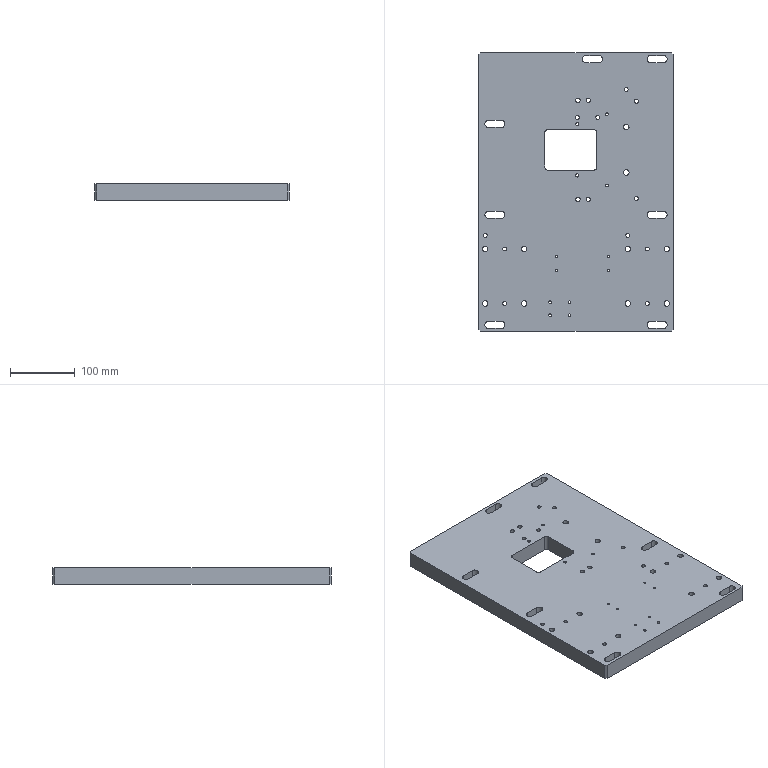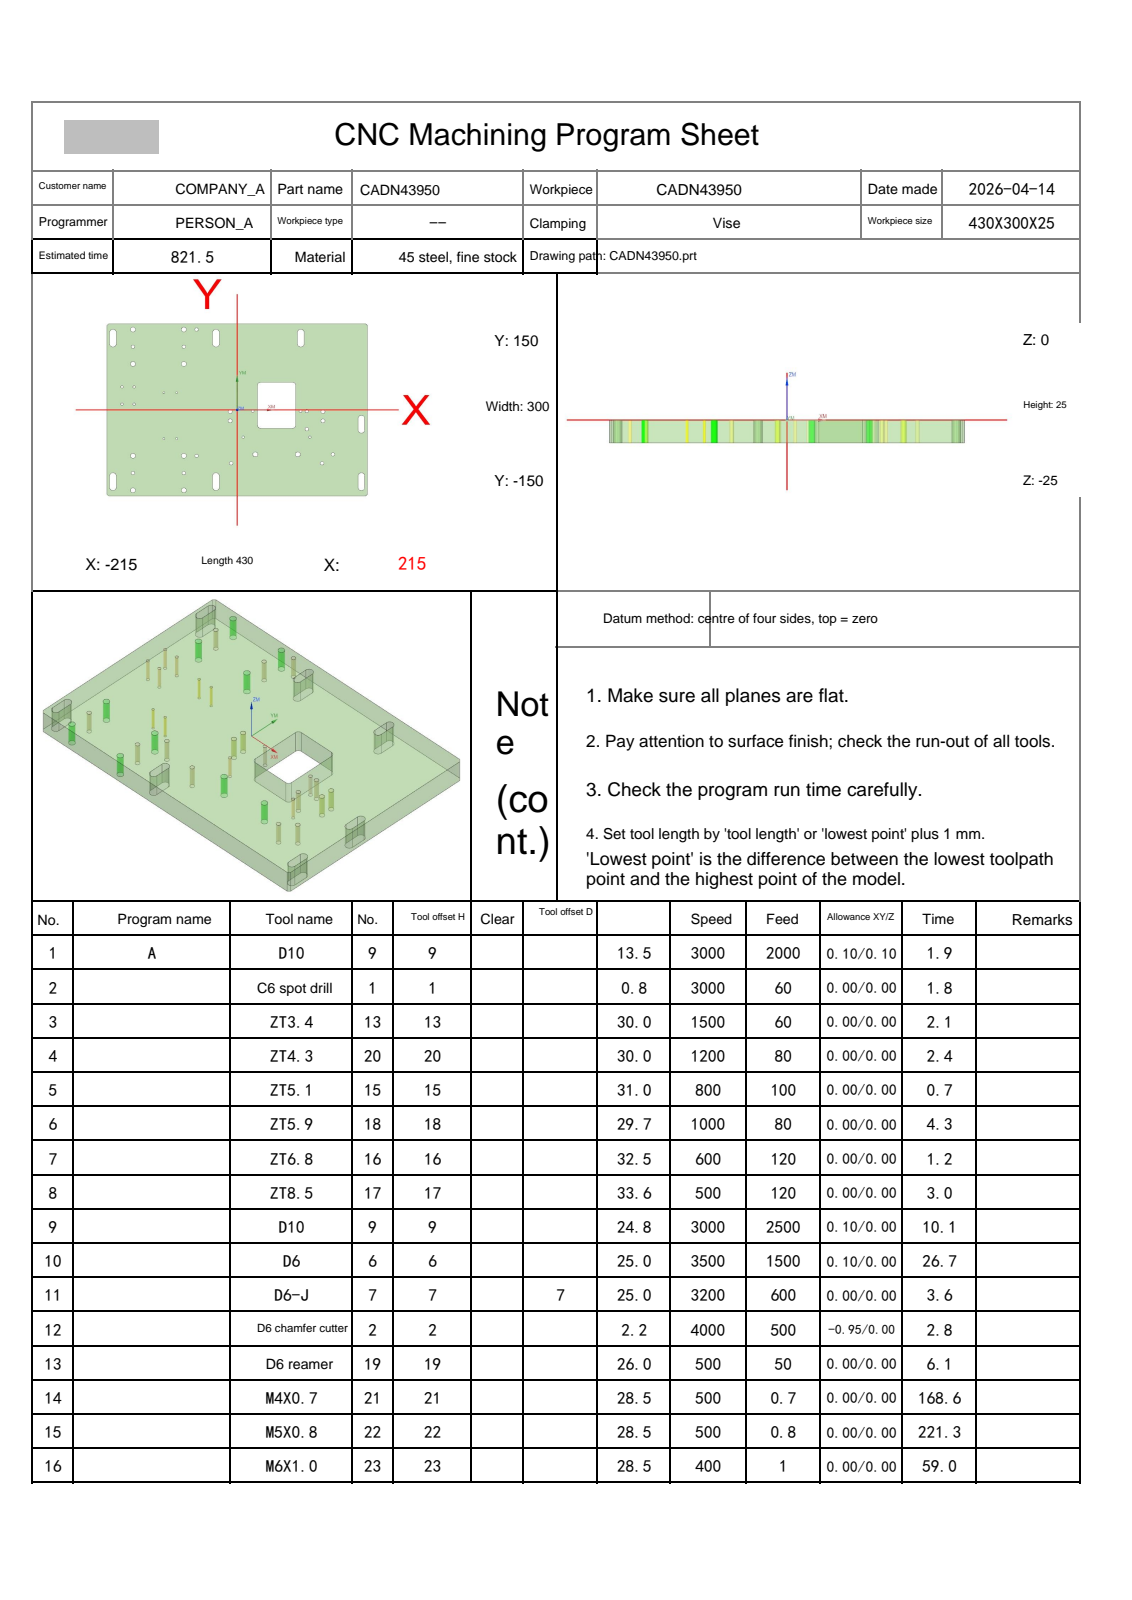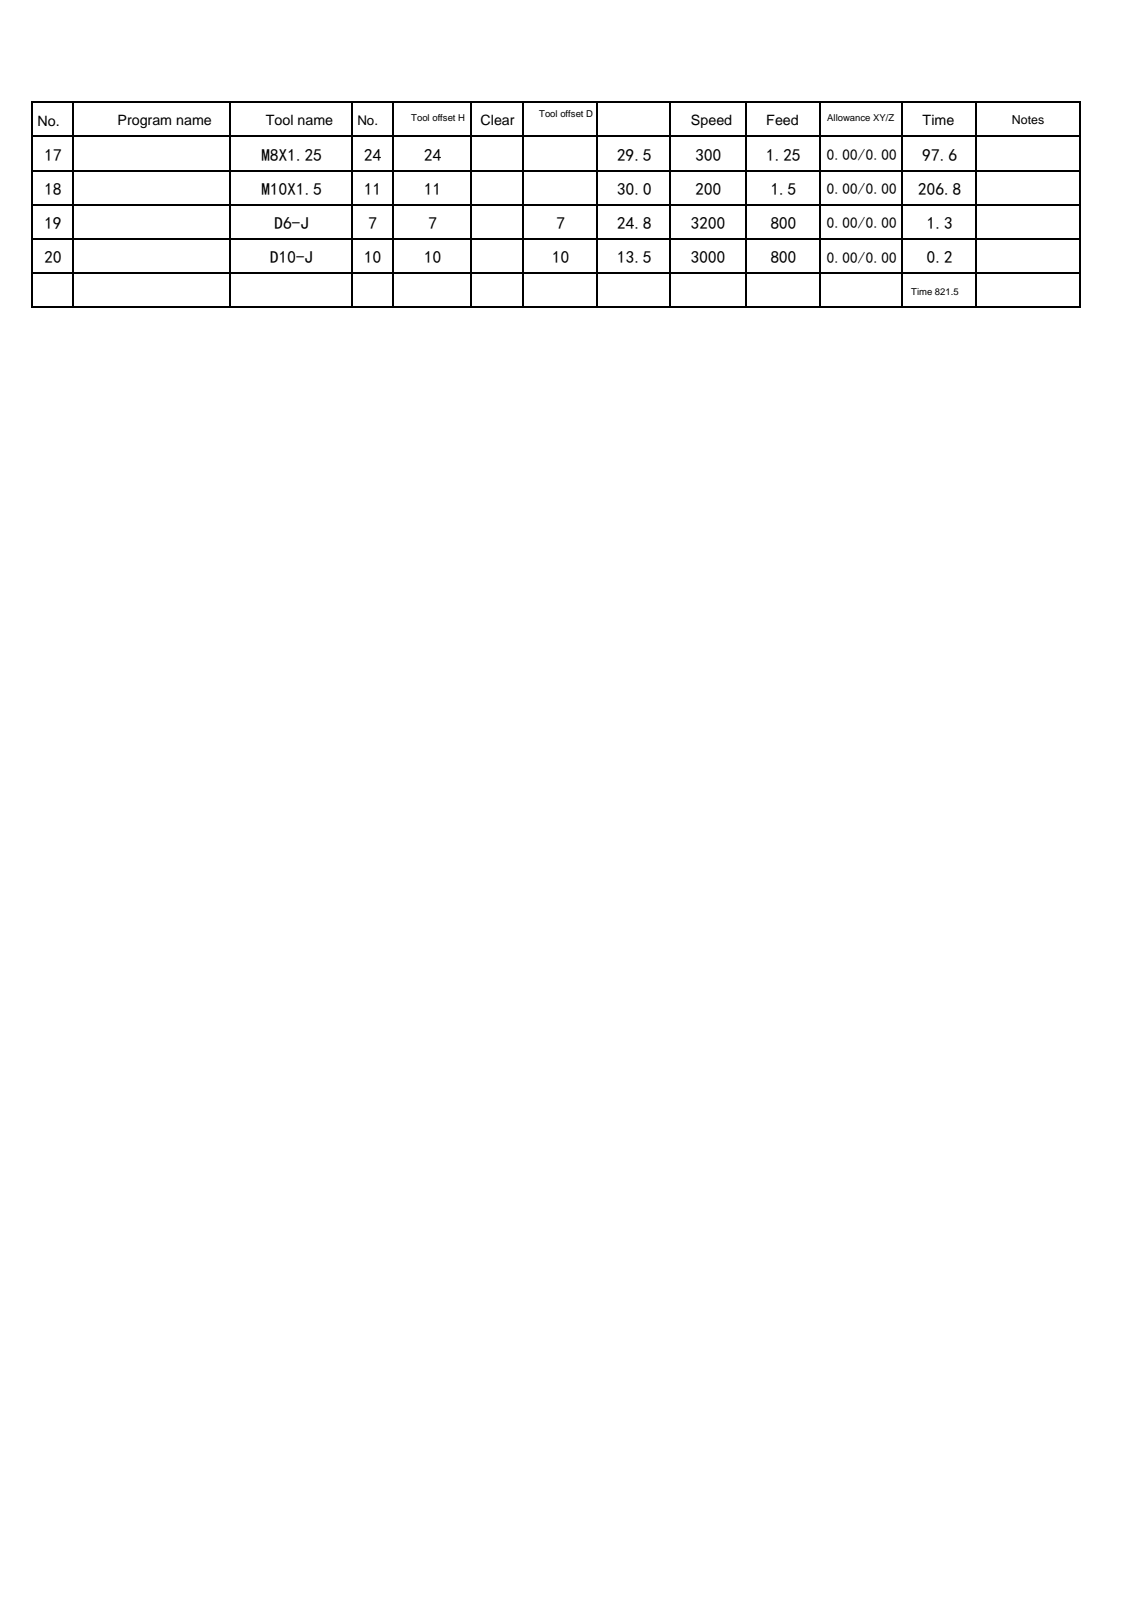NC program | NX | posted by the shop | part box 300 x 430 x 25 mm
Lines 1269 to 2074 of 7024:
N10 T06 M06
(D6  D=6. R=0. H=06 ce=0.10 di=0.00)
G00 G90 G54 X-207.4 Y-125. M03 S3500
G43 H06 Z20.
M08
Z.5
G01 Y-135. Z.455 F1500.
G03 X-205. Y-137.4 Z.438 I2.4 J0.0
X-202.6 Y-135. Z.421 I0.0 J2.4
G01 Y-115. Z.331
G03 X-205. Y-112.6 Z.314 I-2.4 J0.0
X-207.4 Y-115. Z.297 I0.0 J-2.4
G01 Y-135. Z.207
G03 X-205. Y-137.4 Z.191 I2.4 J0.0
X-202.6 Y-135. Z.174 I0.0 J2.4
G01 Y-115. Z.084
G03 X-205. Y-112.6 Z.067 I-2.4 J0.0
X-207.4 Y-115. Z.05 I0.0 J-2.4
G01 Y-135. Z-.04
G03 X-205. Y-137.4 Z-.057 I2.4 J0.0
X-202.6 Y-135. Z-.074 I0.0 J2.4
G01 Y-115. Z-.164
G03 X-205. Y-112.6 Z-.181 I-2.4 J0.0
X-207.4 Y-115. Z-.198 I0.0 J-2.4
G01 Y-135. Z-.288
G03 X-205. Y-137.4 Z-.305 I2.4 J0.0
X-202.6 Y-135. Z-.322 I0.0 J2.4
G01 Y-115. Z-.411
G03 X-205. Y-112.6 Z-.428 I-2.4 J0.0
X-207.4 Y-115. Z-.445 I0.0 J-2.4
G01 Y-135. Z-.535
G03 X-205. Y-137.4 Z-.552 I2.4 J0.0
X-202.6 Y-135. Z-.569 I0.0 J2.4
G01 Y-115. Z-.659
G03 X-205. Y-112.6 Z-.676 I-2.4 J0.0
X-207.4 Y-115. Z-.693 I0.0 J-2.4
G01 Y-135. Z-.783
G03 X-205. Y-137.4 Z-.8 I2.4 J0.0
X-202.6 Y-135. Z-.817 I0.0 J2.4
G01 Y-115. Z-.907
G03 X-205. Y-112.6 Z-.924 I-2.4 J0.0
X-207.4 Y-115. Z-.94 I0.0 J-2.4
G01 Y-135. Z-1.03
G03 X-205. Y-137.4 Z-1.047 I2.4 J0.0
X-202.6 Y-135. Z-1.064 I0.0 J2.4
G01 Y-115. Z-1.154
G03 X-205. Y-112.6 Z-1.171 I-2.4 J0.0
X-207.4 Y-115. Z-1.188 I0.0 J-2.4
G01 Y-135. Z-1.278
G03 X-205. Y-137.4 Z-1.295 I2.4 J0.0
X-202.6 Y-135. Z-1.312 I0.0 J2.4
G01 Y-115. Z-1.402
G03 X-205. Y-112.6 Z-1.419 I-2.4 J0.0
X-207.4 Y-115. Z-1.436 I0.0 J-2.4
G01 Y-135. Z-1.526
G03 X-205. Y-137.4 Z-1.542 I2.4 J0.0
X-202.6 Y-135. Z-1.559 I0.0 J2.4
G01 Y-115. Z-1.649
G03 X-205. Y-112.6 Z-1.666 I-2.4 J0.0
X-207.4 Y-115. Z-1.683 I0.0 J-2.4
G01 Y-135. Z-1.773
G03 X-205. Y-137.4 Z-1.79 I2.4 J0.0
X-202.6 Y-135. Z-1.807 I0.0 J2.4
G01 Y-115. Z-1.897
G03 X-205. Y-112.6 Z-1.914 I-2.4 J0.0
X-207.4 Y-115. Z-1.931 I0.0 J-2.4
G01 Y-135. Z-2.021
G03 X-205. Y-137.4 Z-2.038 I2.4 J0.0
X-202.6 Y-135. Z-2.055 I0.0 J2.4
G01 Y-115. Z-2.144
G03 X-205. Y-112.6 Z-2.161 I-2.4 J0.0
X-207.4 Y-115. Z-2.178 I0.0 J-2.4
G01 Y-135. Z-2.268
G03 X-205. Y-137.4 Z-2.285 I2.4 J0.0
X-202.6 Y-135. Z-2.302 I0.0 J2.4
G01 Y-115. Z-2.392
G03 X-205. Y-112.6 Z-2.409 I-2.4 J0.0
X-207.4 Y-115. Z-2.426 I0.0 J-2.4
G01 Y-135. Z-2.516
G03 X-205. Y-137.4 Z-2.533 I2.4 J0.0
X-202.6 Y-135. Z-2.55 I0.0 J2.4
G01 Y-115. Z-2.64
G03 X-205. Y-112.6 Z-2.657 I-2.4 J0.0
X-207.4 Y-115. Z-2.673 I0.0 J-2.4
G01 Y-135. Z-2.763
G03 X-205. Y-137.4 Z-2.78 I2.4 J0.0
X-202.6 Y-135. Z-2.797 I0.0 J2.4
G01 Y-115. Z-2.887
G03 X-205. Y-112.6 Z-2.904 I-2.4 J0.0
X-207.4 Y-115. Z-2.921 I0.0 J-2.4
G01 Y-135. Z-3.011
G03 X-205. Y-137.4 Z-3.028 I2.4 J0.0
X-202.6 Y-135. Z-3.045 I0.0 J2.4
G01 Y-115. Z-3.135
G03 X-205. Y-112.6 Z-3.152 I-2.4 J0.0
X-207.4 Y-115. Z-3.169 I0.0 J-2.4
G01 Y-135. Z-3.259
G03 X-205. Y-137.4 Z-3.275 I2.4 J0.0
X-202.6 Y-135. Z-3.292 I0.0 J2.4
G01 Y-115. Z-3.382
G03 X-205. Y-112.6 Z-3.399 I-2.4 J0.0
X-207.4 Y-115. Z-3.416 I0.0 J-2.4
G01 Y-135. Z-3.506
G03 X-205. Y-137.4 Z-3.523 I2.4 J0.0
X-202.6 Y-135. Z-3.54 I0.0 J2.4
G01 Y-115. Z-3.63
G03 X-205. Y-112.6 Z-3.647 I-2.4 J0.0
X-207.4 Y-115. Z-3.664 I0.0 J-2.4
G01 Y-135. Z-3.754
G03 X-205. Y-137.4 Z-3.771 I2.4 J0.0
X-202.6 Y-135. Z-3.788 I0.0 J2.4
G01 Y-115. Z-3.877
G03 X-205. Y-112.6 Z-3.894 I-2.4 J0.0
X-207.4 Y-115. Z-3.911 I0.0 J-2.4
G01 Y-135. Z-4.001
G03 X-205. Y-137.4 Z-4.018 I2.4 J0.0
X-202.6 Y-135. Z-4.035 I0.0 J2.4
G01 Y-115. Z-4.125
G03 X-205. Y-112.6 Z-4.142 I-2.4 J0.0
X-207.4 Y-115. Z-4.159 I0.0 J-2.4
G01 Y-135. Z-4.249
G03 X-205. Y-137.4 Z-4.266 I2.4 J0.0
X-202.6 Y-135. Z-4.283 I0.0 J2.4
G01 Y-115. Z-4.373
G03 X-205. Y-112.6 Z-4.39 I-2.4 J0.0
X-207.4 Y-115. Z-4.407 I0.0 J-2.4
G01 Y-135. Z-4.496
G03 X-205. Y-137.4 Z-4.513 I2.4 J0.0
X-202.6 Y-135. Z-4.53 I0.0 J2.4
G01 Y-115. Z-4.62
G03 X-205. Y-112.6 Z-4.637 I-2.4 J0.0
X-207.4 Y-115. Z-4.654 I0.0 J-2.4
G01 Y-135. Z-4.744
G03 X-205. Y-137.4 Z-4.761 I2.4 J0.0
X-202.6 Y-135. Z-4.778 I0.0 J2.4
G01 Y-115. Z-4.868
G03 X-205. Y-112.6 Z-4.885 I-2.4 J0.0
X-207.4 Y-115. Z-4.902 I0.0 J-2.4
G01 Y-135. Z-4.992
G03 X-205. Y-137.4 Z-5.008 I2.4 J0.0
X-202.6 Y-135. Z-5.025 I0.0 J2.4
G01 Y-115. Z-5.115
G03 X-205. Y-112.6 Z-5.132 I-2.4 J0.0
X-207.4 Y-115. Z-5.149 I0.0 J-2.4
G01 Y-135. Z-5.239
G03 X-205. Y-137.4 Z-5.256 I2.4 J0.0
X-202.6 Y-135. Z-5.273 I0.0 J2.4
G01 Y-115. Z-5.363
G03 X-205. Y-112.6 Z-5.38 I-2.4 J0.0
X-207.4 Y-115. Z-5.397 I0.0 J-2.4
G01 Y-135. Z-5.487
G03 X-205. Y-137.4 Z-5.504 I2.4 J0.0
X-202.6 Y-135. Z-5.521 I0.0 J2.4
G01 Y-115. Z-5.61
G03 X-205. Y-112.6 Z-5.627 I-2.4 J0.0
X-207.4 Y-115. Z-5.644 I0.0 J-2.4
G01 Y-135. Z-5.734
G03 X-205. Y-137.4 Z-5.751 I2.4 J0.0
X-202.6 Y-135. Z-5.768 I0.0 J2.4
G01 Y-115. Z-5.858
G03 X-205. Y-112.6 Z-5.875 I-2.4 J0.0
X-207.4 Y-115. Z-5.892 I0.0 J-2.4
G01 Y-135. Z-5.982
G03 X-205. Y-137.4 Z-5.999 I2.4 J0.0
X-202.6 Y-135. Z-6.016 I0.0 J2.4
G01 Y-115. Z-6.106
G03 X-205. Y-112.6 Z-6.123 I-2.4 J0.0
X-207.4 Y-115. Z-6.14 I0.0 J-2.4
G01 Y-135. Z-6.229
G03 X-205. Y-137.4 Z-6.246 I2.4 J0.0
X-202.6 Y-135. Z-6.263 I0.0 J2.4
G01 Y-115. Z-6.353
G03 X-205. Y-112.6 Z-6.37 I-2.4 J0.0
X-207.4 Y-115. Z-6.387 I0.0 J-2.4
G01 Y-135. Z-6.477
G03 X-205. Y-137.4 Z-6.494 I2.4 J0.0
X-202.6 Y-135. Z-6.511 I0.0 J2.4
G01 Y-115. Z-6.601
G03 X-205. Y-112.6 Z-6.618 I-2.4 J0.0
X-207.4 Y-115. Z-6.635 I0.0 J-2.4
G01 Y-135. Z-6.725
G03 X-205. Y-137.4 Z-6.742 I2.4 J0.0
X-202.6 Y-135. Z-6.758 I0.0 J2.4
G01 Y-115. Z-6.848
G03 X-205. Y-112.6 Z-6.865 I-2.4 J0.0
X-207.4 Y-115. Z-6.882 I0.0 J-2.4
G01 Y-135. Z-6.972
G03 X-205. Y-137.4 Z-6.989 I2.4 J0.0
X-202.6 Y-135. Z-7.006 I0.0 J2.4
G01 Y-115. Z-7.096
G03 X-205. Y-112.6 Z-7.113 I-2.4 J0.0
X-207.4 Y-115. Z-7.13 I0.0 J-2.4
G01 Y-135. Z-7.22
G03 X-205. Y-137.4 Z-7.237 I2.4 J0.0
X-202.6 Y-135. Z-7.254 I0.0 J2.4
G01 Y-115. Z-7.343
G03 X-205. Y-112.6 Z-7.36 I-2.4 J0.0
X-207.4 Y-115. Z-7.377 I0.0 J-2.4
G01 Y-135. Z-7.467
G03 X-205. Y-137.4 Z-7.484 I2.4 J0.0
X-202.6 Y-135. Z-7.501 I0.0 J2.4
G01 Y-115. Z-7.591
G03 X-205. Y-112.6 Z-7.608 I-2.4 J0.0
X-207.4 Y-115. Z-7.625 I0.0 J-2.4
G01 Y-135. Z-7.715
G03 X-205. Y-137.4 Z-7.732 I2.4 J0.0
X-202.6 Y-135. Z-7.749 I0.0 J2.4
G01 Y-115. Z-7.839
G03 X-205. Y-112.6 Z-7.856 I-2.4 J0.0
X-207.4 Y-115. Z-7.873 I0.0 J-2.4
G01 Y-135. Z-7.962
G03 X-205. Y-137.4 Z-7.979 I2.4 J0.0
X-202.6 Y-135. Z-7.996 I0.0 J2.4
G01 Y-115. Z-8.086
G03 X-205. Y-112.6 Z-8.103 I-2.4 J0.0
X-207.4 Y-115. Z-8.12 I0.0 J-2.4
G01 Y-135. Z-8.21
G03 X-205. Y-137.4 Z-8.227 I2.4 J0.0
X-202.6 Y-135. Z-8.244 I0.0 J2.4
G01 Y-115. Z-8.334
G03 X-205. Y-112.6 Z-8.351 I-2.4 J0.0
X-207.4 Y-115. Z-8.368 I0.0 J-2.4
G01 Y-135. Z-8.458
G03 X-205. Y-137.4 Z-8.475 I2.4 J0.0
X-202.6 Y-135. Z-8.491 I0.0 J2.4
G01 Y-115. Z-8.581
G03 X-205. Y-112.6 Z-8.598 I-2.4 J0.0
X-207.4 Y-115. Z-8.615 I0.0 J-2.4
G01 Y-135. Z-8.705
G03 X-205. Y-137.4 Z-8.722 I2.4 J0.0
X-202.6 Y-135. Z-8.739 I0.0 J2.4
G01 Y-115. Z-8.829
G03 X-205. Y-112.6 Z-8.846 I-2.4 J0.0
X-207.4 Y-115. Z-8.863 I0.0 J-2.4
G01 Y-135. Z-8.953
G03 X-205. Y-137.4 Z-8.97 I2.4 J0.0
X-202.6 Y-135. Z-8.987 I0.0 J2.4
G01 Y-115. Z-9.077
G03 X-205. Y-112.6 Z-9.093 I-2.4 J0.0
X-207.4 Y-115. Z-9.11 I0.0 J-2.4
G01 Y-135. Z-9.2
G03 X-205. Y-137.4 Z-9.217 I2.4 J0.0
X-202.6 Y-135. Z-9.234 I0.0 J2.4
G01 Y-115. Z-9.324
G03 X-205. Y-112.6 Z-9.341 I-2.4 J0.0
X-207.4 Y-115. Z-9.358 I0.0 J-2.4
G01 Y-135. Z-9.448
G03 X-205. Y-137.4 Z-9.465 I2.4 J0.0
X-202.6 Y-135. Z-9.482 I0.0 J2.4
G01 Y-115. Z-9.572
G03 X-205. Y-112.6 Z-9.589 I-2.4 J0.0
X-207.4 Y-115. Z-9.606 I0.0 J-2.4
G01 Y-135. Z-9.695
G03 X-205. Y-137.4 Z-9.712 I2.4 J0.0
X-202.6 Y-135. Z-9.729 I0.0 J2.4
G01 Y-115. Z-9.819
G03 X-205. Y-112.6 Z-9.836 I-2.4 J0.0
X-207.4 Y-115. Z-9.853 I0.0 J-2.4
G01 Y-135. Z-9.943
G03 X-205. Y-137.4 Z-9.96 I2.4 J0.0
X-202.6 Y-135. Z-9.977 I0.0 J2.4
G01 Y-115. Z-10.067
G03 X-205. Y-112.6 Z-10.084 I-2.4 J0.0
X-207.4 Y-115. Z-10.101 I0.0 J-2.4
G01 Y-135. Z-10.191
G03 X-205. Y-137.4 Z-10.208 I2.4 J0.0
X-202.6 Y-135. Z-10.224 I0.0 J2.4
G01 Y-115. Z-10.314
G03 X-205. Y-112.6 Z-10.331 I-2.4 J0.0
X-207.4 Y-115. Z-10.348 I0.0 J-2.4
G01 Y-135. Z-10.438
G03 X-205. Y-137.4 Z-10.455 I2.4 J0.0
X-202.6 Y-135. Z-10.472 I0.0 J2.4
G01 Y-115. Z-10.562
G03 X-205. Y-112.6 Z-10.579 I-2.4 J0.0
X-207.4 Y-115. Z-10.596 I0.0 J-2.4
G01 Y-135. Z-10.686
G03 X-205. Y-137.4 Z-10.703 I2.4 J0.0
X-202.6 Y-135. Z-10.72 I0.0 J2.4
G01 Y-115. Z-10.81
G03 X-205. Y-112.6 Z-10.826 I-2.4 J0.0
X-207.4 Y-115. Z-10.843 I0.0 J-2.4
G01 Y-135. Z-10.933
G03 X-205. Y-137.4 Z-10.95 I2.4 J0.0
X-202.6 Y-135. Z-10.967 I0.0 J2.4
G01 Y-115. Z-11.057
G03 X-205. Y-112.6 Z-11.074 I-2.4 J0.0
X-207.4 Y-115. Z-11.091 I0.0 J-2.4
G01 Y-135. Z-11.181
G03 X-205. Y-137.4 Z-11.198 I2.4 J0.0
X-202.6 Y-135. Z-11.215 I0.0 J2.4
G01 Y-115. Z-11.305
G03 X-205. Y-112.6 Z-11.322 I-2.4 J0.0
X-207.4 Y-115. Z-11.339 I0.0 J-2.4
G01 Y-135. Z-11.428
G03 X-205. Y-137.4 Z-11.445 I2.4 J0.0
X-202.6 Y-135. Z-11.462 I0.0 J2.4
G01 Y-115. Z-11.552
G03 X-205. Y-112.6 Z-11.569 I-2.4 J0.0
X-207.4 Y-115. Z-11.586 I0.0 J-2.4
G01 Y-135. Z-11.676
G03 X-205. Y-137.4 Z-11.693 I2.4 J0.0
X-202.6 Y-135. Z-11.71 I0.0 J2.4
G01 Y-115. Z-11.8
G03 X-205. Y-112.6 Z-11.817 I-2.4 J0.0
X-207.4 Y-115. Z-11.834 I0.0 J-2.4
G01 Y-135. Z-11.924
G03 X-205. Y-137.4 Z-11.941 I2.4 J0.0
X-202.6 Y-135. Z-11.957 I0.0 J2.4
G01 Y-115. Z-12.047
G03 X-205. Y-112.6 Z-12.064 I-2.4 J0.0
X-207.4 Y-115. Z-12.081 I0.0 J-2.4
G01 Y-135. Z-12.171
G03 X-205. Y-137.4 Z-12.188 I2.4 J0.0
X-202.6 Y-135. Z-12.205 I0.0 J2.4
G01 Y-115. Z-12.295
G03 X-205. Y-112.6 Z-12.312 I-2.4 J0.0
X-207.4 Y-115. Z-12.329 I0.0 J-2.4
G01 Y-135. Z-12.419
G03 X-205. Y-137.4 Z-12.436 I2.4 J0.0
X-202.6 Y-135. Z-12.453 I0.0 J2.4
G01 Y-115. Z-12.543
G03 X-205. Y-112.6 Z-12.559 I-2.4 J0.0
X-207.4 Y-115. Z-12.576 I0.0 J-2.4
G01 Y-135. Z-12.666
G03 X-205. Y-137.4 Z-12.683 I2.4 J0.0
X-202.6 Y-135. Z-12.7 I0.0 J2.4
G01 Y-115. Z-12.79
G03 X-205. Y-112.6 Z-12.807 I-2.4 J0.0
X-207.4 Y-115. Z-12.824 I0.0 J-2.4
G01 Y-135. Z-12.914
G03 X-205. Y-137.4 Z-12.931 I2.4 J0.0
X-202.6 Y-135. Z-12.948 I0.0 J2.4
G01 Y-115. Z-13.038
G03 X-205. Y-112.6 Z-13.055 I-2.4 J0.0
X-207.4 Y-115. Z-13.072 I0.0 J-2.4
G01 Y-135. Z-13.161
G03 X-205. Y-137.4 Z-13.178 I2.4 J0.0
X-202.6 Y-135. Z-13.195 I0.0 J2.4
G01 Y-115. Z-13.285
G03 X-205. Y-112.6 Z-13.302 I-2.4 J0.0
X-207.4 Y-115. Z-13.319 I0.0 J-2.4
G01 Y-135. Z-13.409
G03 X-205. Y-137.4 Z-13.426 I2.4 J0.0
X-202.6 Y-135. Z-13.443 I0.0 J2.4
G01 Y-115. Z-13.533
G03 X-205. Y-112.6 Z-13.55 I-2.4 J0.0
X-207.4 Y-115. Z-13.567 I0.0 J-2.4
G01 Y-135. Z-13.657
G03 X-205. Y-137.4 Z-13.674 I2.4 J0.0
X-202.6 Y-135. Z-13.69 I0.0 J2.4
G01 Y-115. Z-13.78
G03 X-205. Y-112.6 Z-13.797 I-2.4 J0.0
X-207.4 Y-115. Z-13.814 I0.0 J-2.4
G01 Y-135. Z-13.904
G03 X-205. Y-137.4 Z-13.921 I2.4 J0.0
X-202.6 Y-135. Z-13.938 I0.0 J2.4
G01 Y-115. Z-14.028
G03 X-205. Y-112.6 Z-14.045 I-2.4 J0.0
X-207.4 Y-115. Z-14.062 I0.0 J-2.4
G01 Y-135. Z-14.152
G03 X-205. Y-137.4 Z-14.169 I2.4 J0.0
X-202.6 Y-135. Z-14.186 I0.0 J2.4
G01 Y-115. Z-14.276
G03 X-205. Y-112.6 Z-14.292 I-2.4 J0.0
X-207.4 Y-115. Z-14.309 I0.0 J-2.4
G01 Y-135. Z-14.399
G03 X-205. Y-137.4 Z-14.416 I2.4 J0.0
X-202.6 Y-135. Z-14.433 I0.0 J2.4
G01 Y-115. Z-14.523
G03 X-205. Y-112.6 Z-14.54 I-2.4 J0.0
X-207.4 Y-115. Z-14.557 I0.0 J-2.4
G01 Y-135. Z-14.647
G03 X-205. Y-137.4 Z-14.664 I2.4 J0.0
X-202.6 Y-135. Z-14.681 I0.0 J2.4
G01 Y-115. Z-14.771
G03 X-205. Y-112.6 Z-14.788 I-2.4 J0.0
X-207.4 Y-115. Z-14.805 I0.0 J-2.4
G01 Y-135. Z-14.894
G03 X-205. Y-137.4 Z-14.911 I2.4 J0.0
X-202.6 Y-135. Z-14.928 I0.0 J2.4
G01 Y-115. Z-15.018
G03 X-205. Y-112.6 Z-15.035 I-2.4 J0.0
X-207.4 Y-115. Z-15.052 I0.0 J-2.4
G01 Y-135. Z-15.142
G03 X-205. Y-137.4 Z-15.159 I2.4 J0.0
X-202.6 Y-135. Z-15.176 I0.0 J2.4
G01 Y-115. Z-15.266
G03 X-205. Y-112.6 Z-15.283 I-2.4 J0.0
X-207.4 Y-115. Z-15.3 I0.0 J-2.4
G01 Y-135. Z-15.39
G03 X-205. Y-137.4 Z-15.407 I2.4 J0.0
X-202.6 Y-135. Z-15.423 I0.0 J2.4
G01 Y-115. Z-15.513
G03 X-205. Y-112.6 Z-15.53 I-2.4 J0.0
X-207.4 Y-115. Z-15.547 I0.0 J-2.4
G01 Y-135. Z-15.637
G03 X-205. Y-137.4 Z-15.654 I2.4 J0.0
X-202.6 Y-135. Z-15.671 I0.0 J2.4
G01 Y-115. Z-15.761
G03 X-205. Y-112.6 Z-15.778 I-2.4 J0.0
X-207.4 Y-115. Z-15.795 I0.0 J-2.4
G01 Y-135. Z-15.885
G03 X-205. Y-137.4 Z-15.902 I2.4 J0.0
X-202.6 Y-135. Z-15.919 I0.0 J2.4
G01 Y-115. Z-16.009
G03 X-205. Y-112.6 Z-16.025 I-2.4 J0.0
X-207.4 Y-115. Z-16.042 I0.0 J-2.4
G01 Y-135. Z-16.132
G03 X-205. Y-137.4 Z-16.149 I2.4 J0.0
X-202.6 Y-135. Z-16.166 I0.0 J2.4
G01 Y-115. Z-16.256
G03 X-205. Y-112.6 Z-16.273 I-2.4 J0.0
X-207.4 Y-115. Z-16.29 I0.0 J-2.4
G01 Y-135. Z-16.38
G03 X-205. Y-137.4 Z-16.397 I2.4 J0.0
X-202.6 Y-135. Z-16.414 I0.0 J2.4
G01 Y-115. Z-16.504
G03 X-205. Y-112.6 Z-16.521 I-2.4 J0.0
X-207.4 Y-115. Z-16.538 I0.0 J-2.4
G01 Y-135. Z-16.627
G03 X-205. Y-137.4 Z-16.644 I2.4 J0.0
X-202.6 Y-135. Z-16.661 I0.0 J2.4
G01 Y-115. Z-16.751
G03 X-205. Y-112.6 Z-16.768 I-2.4 J0.0
X-207.4 Y-115. Z-16.785 I0.0 J-2.4
G01 Y-135. Z-16.875
G03 X-205. Y-137.4 Z-16.892 I2.4 J0.0
X-202.6 Y-135. Z-16.909 I0.0 J2.4
G01 Y-115. Z-16.999
G03 X-205. Y-112.6 Z-17.016 I-2.4 J0.0
X-207.4 Y-115. Z-17.033 I0.0 J-2.4
G01 Y-135. Z-17.123
G03 X-205. Y-137.4 Z-17.14 I2.4 J0.0
X-202.6 Y-135. Z-17.157 I0.0 J2.4
G01 Y-115. Z-17.246
G03 X-205. Y-112.6 Z-17.263 I-2.4 J0.0
X-207.4 Y-115. Z-17.28 I0.0 J-2.4
G01 Y-135. Z-17.37
G03 X-205. Y-137.4 Z-17.387 I2.4 J0.0
X-202.6 Y-135. Z-17.404 I0.0 J2.4
G01 Y-115. Z-17.494
G03 X-205. Y-112.6 Z-17.511 I-2.4 J0.0
X-207.4 Y-115. Z-17.528 I0.0 J-2.4
G01 Y-135. Z-17.618
G03 X-205. Y-137.4 Z-17.635 I2.4 J0.0
X-202.6 Y-135. Z-17.652 I0.0 J2.4
G01 Y-115. Z-17.742
G03 X-205. Y-112.6 Z-17.758 I-2.4 J0.0
X-207.4 Y-115. Z-17.775 I0.0 J-2.4
G01 Y-135. Z-17.865
G03 X-205. Y-137.4 Z-17.882 I2.4 J0.0
X-202.6 Y-135. Z-17.899 I0.0 J2.4
G01 Y-115. Z-17.989
G03 X-205. Y-112.6 Z-18.006 I-2.4 J0.0
X-207.4 Y-115. Z-18.023 I0.0 J-2.4
G01 Y-135. Z-18.113
G03 X-205. Y-137.4 Z-18.13 I2.4 J0.0
X-202.6 Y-135. Z-18.147 I0.0 J2.4
G01 Y-115. Z-18.237
G03 X-205. Y-112.6 Z-18.254 I-2.4 J0.0
X-207.4 Y-115. Z-18.271 I0.0 J-2.4
G01 Y-135. Z-18.36
G03 X-205. Y-137.4 Z-18.377 I2.4 J0.0
X-202.6 Y-135. Z-18.394 I0.0 J2.4
G01 Y-115. Z-18.484
G03 X-205. Y-112.6 Z-18.501 I-2.4 J0.0
X-207.4 Y-115. Z-18.518 I0.0 J-2.4
G01 Y-135. Z-18.608
G03 X-205. Y-137.4 Z-18.625 I2.4 J0.0
X-202.6 Y-135. Z-18.642 I0.0 J2.4
G01 Y-115. Z-18.732
G03 X-205. Y-112.6 Z-18.749 I-2.4 J0.0
X-207.4 Y-115. Z-18.766 I0.0 J-2.4
G01 Y-135. Z-18.856
G03 X-205. Y-137.4 Z-18.873 I2.4 J0.0
X-202.6 Y-135. Z-18.89 I0.0 J2.4
G01 Y-115. Z-18.979
G03 X-205. Y-112.6 Z-18.996 I-2.4 J0.0
X-207.4 Y-115. Z-19.013 I0.0 J-2.4
G01 Y-135. Z-19.103
G03 X-205. Y-137.4 Z-19.12 I2.4 J0.0
X-202.6 Y-135. Z-19.137 I0.0 J2.4
G01 Y-115. Z-19.227
G03 X-205. Y-112.6 Z-19.244 I-2.4 J0.0
X-207.4 Y-115. Z-19.261 I0.0 J-2.4
G01 Y-135. Z-19.351
G03 X-205. Y-137.4 Z-19.368 I2.4 J0.0
X-202.6 Y-135. Z-19.385 I0.0 J2.4
G01 Y-115. Z-19.475
G03 X-205. Y-112.6 Z-19.492 I-2.4 J0.0
X-207.4 Y-115. Z-19.508 I0.0 J-2.4
G01 Y-135. Z-19.598
G03 X-205. Y-137.4 Z-19.615 I2.4 J0.0
X-202.6 Y-135. Z-19.632 I0.0 J2.4
G01 Y-115. Z-19.722
G03 X-205. Y-112.6 Z-19.739 I-2.4 J0.0
X-207.4 Y-115. Z-19.756 I0.0 J-2.4
G01 Y-135. Z-19.846
G03 X-205. Y-137.4 Z-19.863 I2.4 J0.0
X-202.6 Y-135. Z-19.88 I0.0 J2.4
G01 Y-115. Z-19.97
G03 X-205. Y-112.6 Z-19.987 I-2.4 J0.0
X-207.4 Y-115. Z-20.004 I0.0 J-2.4
G01 Y-135. Z-20.093
G03 X-205. Y-137.4 Z-20.11 I2.4 J0.0
X-202.6 Y-135. Z-20.127 I0.0 J2.4
G01 Y-115. Z-20.217
G03 X-205. Y-112.6 Z-20.234 I-2.4 J0.0
X-207.4 Y-115. Z-20.251 I0.0 J-2.4
G01 Y-135. Z-20.341
G03 X-205. Y-137.4 Z-20.358 I2.4 J0.0
X-202.6 Y-135. Z-20.375 I0.0 J2.4
G01 Y-115. Z-20.465
G03 X-205. Y-112.6 Z-20.482 I-2.4 J0.0
X-207.4 Y-115. Z-20.499 I0.0 J-2.4
G01 Y-135. Z-20.589
G03 X-205. Y-137.4 Z-20.606 I2.4 J0.0
X-202.6 Y-135. Z-20.623 I0.0 J2.4
G01 Y-115. Z-20.712
G03 X-205. Y-112.6 Z-20.729 I-2.4 J0.0
X-207.4 Y-115. Z-20.746 I0.0 J-2.4
G01 Y-135. Z-20.836
G03 X-205. Y-137.4 Z-20.853 I2.4 J0.0
X-202.6 Y-135. Z-20.87 I0.0 J2.4
G01 Y-115. Z-20.96
G03 X-205. Y-112.6 Z-20.977 I-2.4 J0.0
X-207.4 Y-115. Z-20.994 I0.0 J-2.4
G01 Y-135. Z-21.084
G03 X-205. Y-137.4 Z-21.101 I2.4 J0.0
X-202.6 Y-135. Z-21.118 I0.0 J2.4
G01 Y-115. Z-21.208
G03 X-205. Y-112.6 Z-21.225 I-2.4 J0.0
X-207.4 Y-115. Z-21.241 I0.0 J-2.4
G01 Y-135. Z-21.331
G03 X-205. Y-137.4 Z-21.348 I2.4 J0.0
X-202.6 Y-135. Z-21.365 I0.0 J2.4
G01 Y-115. Z-21.455
G03 X-205. Y-112.6 Z-21.472 I-2.4 J0.0
X-207.4 Y-115. Z-21.489 I0.0 J-2.4
G01 Y-135. Z-21.579
G03 X-205. Y-137.4 Z-21.596 I2.4 J0.0
X-202.6 Y-135. Z-21.613 I0.0 J2.4
G01 Y-115. Z-21.703
G03 X-205. Y-112.6 Z-21.72 I-2.4 J0.0
X-207.4 Y-115. Z-21.737 I0.0 J-2.4
G01 Y-135. Z-21.827
G03 X-205. Y-137.4 Z-21.843 I2.4 J0.0
X-202.6 Y-135. Z-21.86 I0.0 J2.4
G01 Y-115. Z-21.95
G03 X-205. Y-112.6 Z-21.967 I-2.4 J0.0
X-207.4 Y-115. Z-21.984 I0.0 J-2.4
G01 Y-135. Z-22.074
G03 X-205. Y-137.4 Z-22.091 I2.4 J0.0
X-202.6 Y-135. Z-22.108 I0.0 J2.4
G01 Y-115. Z-22.198
G03 X-205. Y-112.6 Z-22.215 I-2.4 J0.0
X-207.4 Y-115. Z-22.232 I0.0 J-2.4
G01 Y-135. Z-22.322
G03 X-205. Y-137.4 Z-22.339 I2.4 J0.0
X-202.6 Y-135. Z-22.356 I0.0 J2.4
G01 Y-115. Z-22.445
G03 X-205. Y-112.6 Z-22.462 I-2.4 J0.0
X-207.4 Y-115. Z-22.479 I0.0 J-2.4
G01 Y-135. Z-22.569
G03 X-205. Y-137.4 Z-22.586 I2.4 J0.0
X-202.6 Y-135. Z-22.603 I0.0 J2.4
G01 Y-115. Z-22.693
G03 X-205. Y-112.6 Z-22.71 I-2.4 J0.0
X-207.4 Y-115. Z-22.727 I0.0 J-2.4
G01 Y-135. Z-22.817
G03 X-205. Y-137.4 Z-22.834 I2.4 J0.0
X-202.6 Y-135. Z-22.851 I0.0 J2.4
G01 Y-115. Z-22.941
G03 X-205. Y-112.6 Z-22.958 I-2.4 J0.0
X-207.4 Y-115. Z-22.974 I0.0 J-2.4
G01 Y-135. Z-23.064
G03 X-205. Y-137.4 Z-23.081 I2.4 J0.0
X-202.6 Y-135. Z-23.098 I0.0 J2.4
G01 Y-115. Z-23.188
G03 X-205. Y-112.6 Z-23.205 I-2.4 J0.0
X-207.4 Y-115. Z-23.222 I0.0 J-2.4
G01 Y-135. Z-23.312
G03 X-205. Y-137.4 Z-23.329 I2.4 J0.0
X-202.6 Y-135. Z-23.346 I0.0 J2.4
G01 Y-115. Z-23.436
G03 X-205. Y-112.6 Z-23.453 I-2.4 J0.0
X-207.4 Y-115. Z-23.47 I0.0 J-2.4
G01 Y-135. Z-23.56
G03 X-205. Y-137.4 Z-23.576 I2.4 J0.0
X-202.6 Y-135. Z-23.593 I0.0 J2.4
G01 Y-115. Z-23.683
G03 X-205. Y-112.6 Z-23.7 I-2.4 J0.0
X-207.4 Y-115. Z-23.717 I0.0 J-2.4
G01 Y-135. Z-23.807
G03 X-205. Y-137.4 Z-23.824 I2.4 J0.0
X-202.6 Y-135. Z-23.841 I0.0 J2.4
G01 Y-115. Z-23.931
G03 X-205. Y-112.6 Z-23.948 I-2.4 J0.0
X-207.4 Y-115. Z-23.965 I0.0 J-2.4
G01 Y-135. Z-24.055
G03 X-205. Y-137.4 Z-24.072 I2.4 J0.0
X-202.6 Y-135. Z-24.089 I0.0 J2.4
G01 Y-115. Z-24.178
G03 X-205. Y-112.6 Z-24.195 I-2.4 J0.0
X-207.4 Y-115. Z-24.212 I0.0 J-2.4
G01 Y-135. Z-24.302
G03 X-205. Y-137.4 Z-24.319 I2.4 J0.0
X-202.6 Y-135. Z-24.336 I0.0 J2.4
G01 Y-115. Z-24.426
G03 X-205. Y-112.6 Z-24.443 I-2.4 J0.0
X-207.4 Y-115. Z-24.46 I0.0 J-2.4
G01 Y-135. Z-24.55
G03 X-205. Y-137.4 Z-24.567 I2.4 J0.0
X-202.6 Y-135. Z-24.584 I0.0 J2.4
G01 Y-115. Z-24.674
G03 X-205. Y-112.6 Z-24.691 I-2.4 J0.0
X-207.4 Y-115. Z-24.707 I0.0 J-2.4
G01 Y-135. Z-24.797
G03 X-205. Y-137.4 Z-24.814 I2.4 J0.0
X-202.6 Y-135. Z-24.831 I0.0 J2.4
G01 Y-115. Z-24.921
G03 X-205. Y-112.6 Z-24.938 I-2.4 J0.0
X-207.4 Y-115. Z-24.955 I0.0 J-2.4
G01 Y-125. Z-25.
Y-135.
G03 X-205. Y-137.4 I2.4 J0.0
X-202.6 Y-135. I0.0 J2.4
G01 Y-115.
G03 X-205. Y-112.6 I-2.4 J0.0
X-207.4 Y-115. I0.0 J-2.4
G01 Y-125.
Y-125.5
Z-24.
G00 Z20.
X-37.4 Y-125.
Z.5
G01 Y-135. Z.455
G03 X-35. Y-137.4 Z.438 I2.4 J0.0
X-32.6 Y-135. Z.421 I0.0 J2.4
G01 Y-115. Z.331
G03 X-35. Y-112.6 Z.314 I-2.4 J0.0
X-37.4 Y-115. Z.297 I0.0 J-2.4
G01 Y-135. Z.207
G03 X-35. Y-137.4 Z.191 I2.4 J0.0
X-32.6 Y-135. Z.174 I0.0 J2.4
G01 Y-115. Z.084
G03 X-35. Y-112.6 Z.067 I-2.4 J0.0
X-37.4 Y-115. Z.05 I0.0 J-2.4
G01 Y-135. Z-.04
G03 X-35. Y-137.4 Z-.057 I2.4 J0.0
X-32.6 Y-135. Z-.074 I0.0 J2.4
G01 Y-115. Z-.164
G03 X-35. Y-112.6 Z-.181 I-2.4 J0.0
X-37.4 Y-115. Z-.198 I0.0 J-2.4
G01 Y-135. Z-.288
G03 X-35. Y-137.4 Z-.305 I2.4 J0.0
X-32.6 Y-135. Z-.322 I0.0 J2.4
G01 Y-115. Z-.411
G03 X-35. Y-112.6 Z-.428 I-2.4 J0.0
X-37.4 Y-115. Z-.445 I0.0 J-2.4
G01 Y-135. Z-.535
G03 X-35. Y-137.4 Z-.552 I2.4 J0.0
X-32.6 Y-135. Z-.569 I0.0 J2.4
G01 Y-115. Z-.659
G03 X-35. Y-112.6 Z-.676 I-2.4 J0.0
X-37.4 Y-115. Z-.693 I0.0 J-2.4
G01 Y-135. Z-.783
G03 X-35. Y-137.4 Z-.8 I2.4 J0.0
X-32.6 Y-135. Z-.817 I0.0 J2.4
G01 Y-115. Z-.907
G03 X-35. Y-112.6 Z-.924 I-2.4 J0.0
X-37.4 Y-115. Z-.94 I0.0 J-2.4
G01 Y-135. Z-1.03
G03 X-35. Y-137.4 Z-1.047 I2.4 J0.0
X-32.6 Y-135. Z-1.064 I0.0 J2.4
G01 Y-115. Z-1.154
G03 X-35. Y-112.6 Z-1.171 I-2.4 J0.0
X-37.4 Y-115. Z-1.188 I0.0 J-2.4
G01 Y-135. Z-1.278
G03 X-35. Y-137.4 Z-1.295 I2.4 J0.0
X-32.6 Y-135. Z-1.312 I0.0 J2.4
G01 Y-115. Z-1.402
G03 X-35. Y-112.6 Z-1.419 I-2.4 J0.0
X-37.4 Y-115. Z-1.436 I0.0 J-2.4
G01 Y-135. Z-1.526
G03 X-35. Y-137.4 Z-1.542 I2.4 J0.0
X-32.6 Y-135. Z-1.559 I0.0 J2.4
G01 Y-115. Z-1.649
G03 X-35. Y-112.6 Z-1.666 I-2.4 J0.0
X-37.4 Y-115. Z-1.683 I0.0 J-2.4
G01 Y-135. Z-1.773
G03 X-35. Y-137.4 Z-1.79 I2.4 J0.0
X-32.6 Y-135. Z-1.807 I0.0 J2.4
G01 Y-115. Z-1.897
G03 X-35. Y-112.6 Z-1.914 I-2.4 J0.0
X-37.4 Y-115. Z-1.931 I0.0 J-2.4
G01 Y-135. Z-2.021
G03 X-35. Y-137.4 Z-2.038 I2.4 J0.0
X-32.6 Y-135. Z-2.055 I0.0 J2.4
G01 Y-115. Z-2.144
G03 X-35. Y-112.6 Z-2.161 I-2.4 J0.0
X-37.4 Y-115. Z-2.178 I0.0 J-2.4
G01 Y-135. Z-2.268
G03 X-35. Y-137.4 Z-2.285 I2.4 J0.0
X-32.6 Y-135. Z-2.302 I0.0 J2.4
G01 Y-115. Z-2.392
G03 X-35. Y-112.6 Z-2.409 I-2.4 J0.0
X-37.4 Y-115. Z-2.426 I0.0 J-2.4
G01 Y-135. Z-2.516
G03 X-35. Y-137.4 Z-2.533 I2.4 J0.0
X-32.6 Y-135. Z-2.55 I0.0 J2.4
G01 Y-115. Z-2.64
G03 X-35. Y-112.6 Z-2.657 I-2.4 J0.0
X-37.4 Y-115. Z-2.673 I0.0 J-2.4
G01 Y-135. Z-2.763
G03 X-35. Y-137.4 Z-2.78 I2.4 J0.0
X-32.6 Y-135. Z-2.797 I0.0 J2.4
G01 Y-115. Z-2.887
G03 X-35. Y-112.6 Z-2.904 I-2.4 J0.0
X-37.4 Y-115. Z-2.921 I0.0 J-2.4
G01 Y-135. Z-3.011
G03 X-35. Y-137.4 Z-3.028 I2.4 J0.0
X-32.6 Y-135. Z-3.045 I0.0 J2.4
G01 Y-115. Z-3.135
G03 X-35. Y-112.6 Z-3.152 I-2.4 J0.0
X-37.4 Y-115. Z-3.169 I0.0 J-2.4
G01 Y-135. Z-3.259
G03 X-35. Y-137.4 Z-3.275 I2.4 J0.0
X-32.6 Y-135. Z-3.292 I0.0 J2.4
G01 Y-115. Z-3.382
G03 X-35. Y-112.6 Z-3.399 I-2.4 J0.0
X-37.4 Y-115. Z-3.416 I0.0 J-2.4
G01 Y-135. Z-3.506
G03 X-35. Y-137.4 Z-3.523 I2.4 J0.0
X-32.6 Y-135. Z-3.54 I0.0 J2.4
G01 Y-115. Z-3.63
G03 X-35. Y-112.6 Z-3.647 I-2.4 J0.0
X-37.4 Y-115. Z-3.664 I0.0 J-2.4
G01 Y-135. Z-3.754
G03 X-35. Y-137.4 Z-3.771 I2.4 J0.0
X-32.6 Y-135. Z-3.788 I0.0 J2.4
G01 Y-115. Z-3.877
G03 X-35. Y-112.6 Z-3.894 I-2.4 J0.0
X-37.4 Y-115. Z-3.911 I0.0 J-2.4
G01 Y-135. Z-4.001
G03 X-35. Y-137.4 Z-4.018 I2.4 J0.0
X-32.6 Y-135. Z-4.035 I0.0 J2.4
G01 Y-115. Z-4.125
G03 X-35. Y-112.6 Z-4.142 I-2.4 J0.0
X-37.4 Y-115. Z-4.159 I0.0 J-2.4
G01 Y-135. Z-4.249
G03 X-35. Y-137.4 Z-4.266 I2.4 J0.0
X-32.6 Y-135. Z-4.283 I0.0 J2.4
G01 Y-115. Z-4.373
G03 X-35. Y-112.6 Z-4.39 I-2.4 J0.0
X-37.4 Y-115. Z-4.407 I0.0 J-2.4
G01 Y-135. Z-4.496
G03 X-35. Y-137.4 Z-4.513 I2.4 J0.0
X-32.6 Y-135. Z-4.53 I0.0 J2.4
G01 Y-115. Z-4.62
G03 X-35. Y-112.6 Z-4.637 I-2.4 J0.0
X-37.4 Y-115. Z-4.654 I0.0 J-2.4
G01 Y-135. Z-4.744
G03 X-35. Y-137.4 Z-4.761 I2.4 J0.0
X-32.6 Y-135. Z-4.778 I0.0 J2.4
G01 Y-115. Z-4.868
G03 X-35. Y-112.6 Z-4.885 I-2.4 J0.0
X-37.4 Y-115. Z-4.902 I0.0 J-2.4
G01 Y-135. Z-4.992
G03 X-35. Y-137.4 Z-5.008 I2.4 J0.0
X-32.6 Y-135. Z-5.025 I0.0 J2.4
G01 Y-115. Z-5.115
G03 X-35. Y-112.6 Z-5.132 I-2.4 J0.0
X-37.4 Y-115. Z-5.149 I0.0 J-2.4
G01 Y-135. Z-5.239
G03 X-35. Y-137.4 Z-5.256 I2.4 J0.0
X-32.6 Y-135. Z-5.273 I0.0 J2.4
G01 Y-115. Z-5.363
G03 X-35. Y-112.6 Z-5.38 I-2.4 J0.0
X-37.4 Y-115. Z-5.397 I0.0 J-2.4
G01 Y-135. Z-5.487
G03 X-35. Y-137.4 Z-5.504 I2.4 J0.0
X-32.6 Y-135. Z-5.521 I0.0 J2.4
G01 Y-115. Z-5.61
G03 X-35. Y-112.6 Z-5.627 I-2.4 J0.0
X-37.4 Y-115. Z-5.644 I0.0 J-2.4
G01 Y-135. Z-5.734
G03 X-35. Y-137.4 Z-5.751 I2.4 J0.0
X-32.6 Y-135. Z-5.768 I0.0 J2.4
G01 Y-115. Z-5.858
G03 X-35. Y-112.6 Z-5.875 I-2.4 J0.0
X-37.4 Y-115. Z-5.892 I0.0 J-2.4
G01 Y-135. Z-5.982
G03 X-35. Y-137.4 Z-5.999 I2.4 J0.0
X-32.6 Y-135. Z-6.016 I0.0 J2.4
G01 Y-115. Z-6.106
G03 X-35. Y-112.6 Z-6.123 I-2.4 J0.0
X-37.4 Y-115. Z-6.14 I0.0 J-2.4
G01 Y-135. Z-6.229
G03 X-35. Y-137.4 Z-6.246 I2.4 J0.0
X-32.6 Y-135. Z-6.263 I0.0 J2.4
G01 Y-115. Z-6.353
G03 X-35. Y-112.6 Z-6.37 I-2.4 J0.0
X-37.4 Y-115. Z-6.387 I0.0 J-2.4
G01 Y-135. Z-6.477